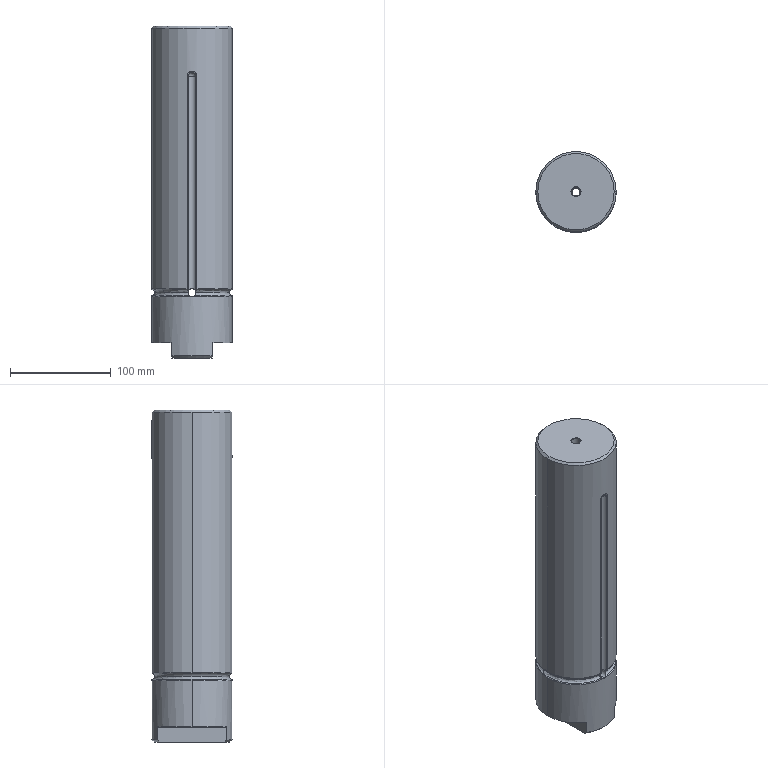Part | SolidWorks | features ICE 5, Fillet 4, 3DProfileFeature 3, HoleWzd 3, Chamfer 2, RevCut 2, Extrusion 1, MirrorPattern 1, RefAxis 1 | 1 solid | 77 faces | box 80 x 80 x 330 mm | volume 1584103 mm3 | cylinder 30 | cone 14 | torus 12 | plane 9 | sphere 6 | spline 6 | commonest cylinder face diameters 8 x10 8.5 x6 2 x4 80 x4 1.6 x2 9 x2